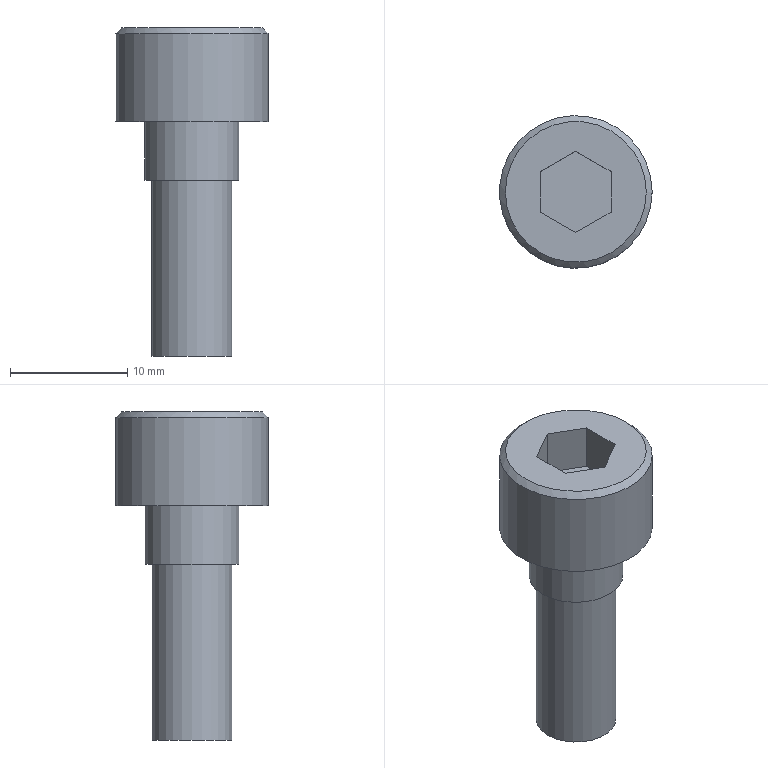Part | STEP file | M3-10_id374_x_t | 1 solid | 15 faces | box 13 x 13 x 28 mm | volume 1728 mm3 | plane 11 | cylinder 3 | cone 1 | commonest cylinder face diameters 6.8 x1 8 x1 13 x1
STEP:
#1=CARTESIAN_POINT('',(-246.986,-112.5,-17.));
#2=VERTEX_POINT('',#1);
#3=CARTESIAN_POINT('',(-243.586,-112.5,-17.));
#4=DIRECTION('',(0.,0.,-1.));
#5=DIRECTION('',(-1.,0.,0.));
#6=AXIS2_PLACEMENT_3D('',#3,#4,#5);
#7=CIRCLE('',#6,3.4);
#8=EDGE_CURVE('',#2,#2,#7,.T.);
#9=ORIENTED_EDGE('',*,*,#8,.F.);
#10=EDGE_LOOP('',(#9));
#11=FACE_BOUND('',#10,.T.);
#12=CARTESIAN_POINT('',(-239.586,-112.5,-17.));
#13=VERTEX_POINT('',#12);
#14=CARTESIAN_POINT('',(-243.586,-112.5,-17.));
#15=DIRECTION('',(0.,0.,1.));
#16=DIRECTION('',(1.,0.,0.));
#17=AXIS2_PLACEMENT_3D('',#14,#15,#16);
#18=CIRCLE('',#17,4.);
#19=EDGE_CURVE('',#13,#13,#18,.T.);
#20=ORIENTED_EDGE('',*,*,#19,.F.);
#21=EDGE_LOOP('',(#20));
#22=FACE_BOUND('',#21,.T.);
#23=CARTESIAN_POINT('',(-243.586,-112.5,-17.));
#24=DIRECTION('',(0.,0.,-1.));
#25=DIRECTION('',(-1.,0.,0.));
#26=AXIS2_PLACEMENT_3D('',#23,#24,#25);
#27=PLANE('',#26);
#28=ADVANCED_FACE('',(#11,#22),#27,.T.);
#29=CARTESIAN_POINT('',(-247.586,-112.5,-12.));
#30=VERTEX_POINT('',#29);
#31=CARTESIAN_POINT('',(-243.586,-112.5,-12.));
#32=DIRECTION('',(0.,0.,1.));
#33=DIRECTION('',(-1.,0.,0.));
#34=AXIS2_PLACEMENT_3D('',#31,#32,#33);
#35=CIRCLE('',#34,4.);
#36=EDGE_CURVE('',#30,#30,#35,.T.);
#37=ORIENTED_EDGE('',*,*,#36,.F.);
#38=EDGE_LOOP('',(#37));
#39=FACE_BOUND('',#38,.T.);
#40=ORIENTED_EDGE('',*,*,#19,.T.);
#41=EDGE_LOOP('',(#40));
#42=FACE_BOUND('',#41,.T.);
#43=CARTESIAN_POINT('',(-243.586,-112.5,-17.));
#44=DIRECTION('',(0.,0.,1.));
#45=DIRECTION('',(1.,0.,0.));
#46=AXIS2_PLACEMENT_3D('',#43,#44,#45);
#47=CYLINDRICAL_SURFACE('',#46,4.);
#48=ADVANCED_FACE('',(#39,#42),#47,.T.);
#49=CARTESIAN_POINT('',(-240.186,-112.5,-32.));
#50=VERTEX_POINT('',#49);
#51=CARTESIAN_POINT('',(-243.586,-112.5,-32.));
#52=DIRECTION('',(0.,0.,1.));
#53=DIRECTION('',(1.,0.,0.));
#54=AXIS2_PLACEMENT_3D('',#51,#52,#53);
#55=CIRCLE('',#54,3.4);
#56=EDGE_CURVE('',#50,#50,#55,.T.);
#57=ORIENTED_EDGE('',*,*,#56,.F.);
#58=EDGE_LOOP('',(#57));
#59=FACE_OUTER_BOUND('',#58,.T.);
#60=CARTESIAN_POINT('',(-243.586,-112.5,-32.));
#61=DIRECTION('',(0.,0.,-1.));
#62=DIRECTION('',(-1.,0.,0.));
#63=AXIS2_PLACEMENT_3D('',#60,#61,#62);
#64=PLANE('',#63);
#65=ADVANCED_FACE('',(#59),#64,.T.);
#66=ORIENTED_EDGE('',*,*,#56,.T.);
#67=EDGE_LOOP('',(#66));
#68=FACE_BOUND('',#67,.T.);
#69=ORIENTED_EDGE('',*,*,#8,.T.);
#70=EDGE_LOOP('',(#69));
#71=FACE_BOUND('',#70,.T.);
#72=CARTESIAN_POINT('',(-243.586,-112.5,-17.));
#73=DIRECTION('',(0.,0.,-1.));
#74=DIRECTION('',(1.,0.,0.));
#75=AXIS2_PLACEMENT_3D('',#72,#73,#74);
#76=CYLINDRICAL_SURFACE('',#75,3.4);
#77=ADVANCED_FACE('',(#68,#71),#76,.T.);
#78=CARTESIAN_POINT('',(-246.586,-110.768,-4.));
#79=VERTEX_POINT('',#78);
#80=CARTESIAN_POINT('',(-246.586,-114.232,-4.));
#81=VERTEX_POINT('',#80);
#82=CARTESIAN_POINT('',(-246.586,-110.768,-4.));
#83=DIRECTION('',(0.,-1.,0.));
#84=VECTOR('',#83,1.);
#85=LINE('',#82,#84);
#86=EDGE_CURVE('',#79,#81,#85,.T.);
#87=ORIENTED_EDGE('',*,*,#86,.F.);
#88=CARTESIAN_POINT('',(-243.586,-109.036,-4.));
#89=VERTEX_POINT('',#88);
#90=CARTESIAN_POINT('',(-243.586,-109.036,-4.));
#91=DIRECTION('',(-0.866,-0.5,0.));
#92=VECTOR('',#91,1.);
#93=LINE('',#90,#92);
#94=EDGE_CURVE('',#89,#79,#93,.T.);
#95=ORIENTED_EDGE('',*,*,#94,.F.);
#96=CARTESIAN_POINT('',(-240.586,-110.768,-4.));
#97=VERTEX_POINT('',#96);
#98=CARTESIAN_POINT('',(-240.586,-110.768,-4.));
#99=DIRECTION('',(-0.866,0.5,0.));
#100=VECTOR('',#99,1.);
#101=LINE('',#98,#100);
#102=EDGE_CURVE('',#97,#89,#101,.T.);
#103=ORIENTED_EDGE('',*,*,#102,.F.);
#104=CARTESIAN_POINT('',(-240.586,-114.232,-4.));
#105=VERTEX_POINT('',#104);
#106=CARTESIAN_POINT('',(-240.586,-114.232,-4.));
#107=DIRECTION('',(0.,1.,0.));
#108=VECTOR('',#107,1.);
#109=LINE('',#106,#108);
#110=EDGE_CURVE('',#105,#97,#109,.T.);
#111=ORIENTED_EDGE('',*,*,#110,.F.);
#112=CARTESIAN_POINT('',(-243.586,-115.964,-4.));
#113=VERTEX_POINT('',#112);
#114=CARTESIAN_POINT('',(-243.586,-115.964,-4.));
#115=DIRECTION('',(0.866,0.5,0.));
#116=VECTOR('',#115,1.);
#117=LINE('',#114,#116);
#118=EDGE_CURVE('',#113,#105,#117,.T.);
#119=ORIENTED_EDGE('',*,*,#118,.F.);
#120=CARTESIAN_POINT('',(-246.586,-114.232,-4.));
#121=DIRECTION('',(0.866,-0.5,0.));
#122=VECTOR('',#121,1.);
#123=LINE('',#120,#122);
#124=EDGE_CURVE('',#81,#113,#123,.T.);
#125=ORIENTED_EDGE('',*,*,#124,.F.);
#126=EDGE_LOOP('',(#87,#95,#103,#111,#119,#125));
#127=FACE_BOUND('',#126,.T.);
#128=CARTESIAN_POINT('',(-237.586,-112.5,-4.));
#129=VERTEX_POINT('',#128);
#130=CARTESIAN_POINT('',(-243.586,-112.5,-4.));
#131=DIRECTION('',(0.,0.,1.));
#132=DIRECTION('',(1.,0.,0.));
#133=AXIS2_PLACEMENT_3D('',#130,#131,#132);
#134=CIRCLE('',#133,6.);
#135=EDGE_CURVE('',#129,#129,#134,.T.);
#136=ORIENTED_EDGE('',*,*,#135,.T.);
#137=EDGE_LOOP('',(#136));
#138=FACE_BOUND('',#137,.T.);
#139=CARTESIAN_POINT('',(-243.586,-112.5,-4.));
#140=DIRECTION('',(0.,0.,1.));
#141=DIRECTION('',(1.,0.,0.));
#142=AXIS2_PLACEMENT_3D('',#139,#140,#141);
#143=PLANE('',#142);
#144=ADVANCED_FACE('',(#127,#138),#143,.T.);
#145=ORIENTED_EDGE('',*,*,#36,.T.);
#146=EDGE_LOOP('',(#145));
#147=FACE_BOUND('',#146,.T.);
#148=CARTESIAN_POINT('',(-237.086,-112.5,-12.));
#149=VERTEX_POINT('',#148);
#150=CARTESIAN_POINT('',(-243.586,-112.5,-12.));
#151=DIRECTION('',(0.,0.,1.));
#152=DIRECTION('',(1.,0.,0.));
#153=AXIS2_PLACEMENT_3D('',#150,#151,#152);
#154=CIRCLE('',#153,6.5);
#155=EDGE_CURVE('',#149,#149,#154,.T.);
#156=ORIENTED_EDGE('',*,*,#155,.F.);
#157=EDGE_LOOP('',(#156));
#158=FACE_BOUND('',#157,.T.);
#159=CARTESIAN_POINT('',(-243.586,-112.5,-12.));
#160=DIRECTION('',(0.,0.,-1.));
#161=DIRECTION('',(-1.,0.,0.));
#162=AXIS2_PLACEMENT_3D('',#159,#160,#161);
#163=PLANE('',#162);
#164=ADVANCED_FACE('',(#147,#158),#163,.T.);
#165=CARTESIAN_POINT('',(-237.086,-112.5,-4.5));
#166=VERTEX_POINT('',#165);
#167=CARTESIAN_POINT('',(-243.586,-112.5,-4.5));
#168=DIRECTION('',(0.,0.,-1.));
#169=DIRECTION('',(1.,0.,0.));
#170=AXIS2_PLACEMENT_3D('',#167,#168,#169);
#171=CIRCLE('',#170,6.5);
#172=EDGE_CURVE('',#166,#166,#171,.T.);
#173=ORIENTED_EDGE('',*,*,#172,.T.);
#174=EDGE_LOOP('',(#173));
#175=FACE_BOUND('',#174,.T.);
#176=ORIENTED_EDGE('',*,*,#155,.T.);
#177=EDGE_LOOP('',(#176));
#178=FACE_BOUND('',#177,.T.);
#179=CARTESIAN_POINT('',(-243.586,-112.5,-12.));
#180=DIRECTION('',(0.,0.,1.));
#181=DIRECTION('',(1.,0.,0.));
#182=AXIS2_PLACEMENT_3D('',#179,#180,#181);
#183=CYLINDRICAL_SURFACE('',#182,6.5);
#184=ADVANCED_FACE('',(#175,#178),#183,.T.);
#185=ORIENTED_EDGE('',*,*,#135,.F.);
#186=EDGE_LOOP('',(#185));
#187=FACE_BOUND('',#186,.T.);
#188=ORIENTED_EDGE('',*,*,#172,.F.);
#189=EDGE_LOOP('',(#188));
#190=FACE_BOUND('',#189,.T.);
#191=CARTESIAN_POINT('',(-243.586,-112.5,-4.5));
#192=DIRECTION('',(0.,0.,-1.));
#193=DIRECTION('',(-1.,0.,0.));
#194=AXIS2_PLACEMENT_3D('',#191,#192,#193);
#195=CONICAL_SURFACE('',#194,6.5,45.);
#196=ADVANCED_FACE('',(#187,#190),#195,.T.);
#197=ORIENTED_EDGE('',*,*,#86,.T.);
#198=CARTESIAN_POINT('',(-246.586,-114.232,-8.));
#199=VERTEX_POINT('',#198);
#200=CARTESIAN_POINT('',(-246.586,-114.232,-8.));
#201=DIRECTION('',(0.,0.,-1.));
#202=VECTOR('',#201,1.);
#203=LINE('',#200,#202);
#204=EDGE_CURVE('',#81,#199,#203,.T.);
#205=ORIENTED_EDGE('',*,*,#204,.T.);
#206=CARTESIAN_POINT('',(-246.586,-110.768,-8.));
#207=VERTEX_POINT('',#206);
#208=CARTESIAN_POINT('',(-246.586,-110.768,-8.));
#209=DIRECTION('',(0.,1.,0.));
#210=VECTOR('',#209,1.);
#211=LINE('',#208,#210);
#212=EDGE_CURVE('',#199,#207,#211,.T.);
#213=ORIENTED_EDGE('',*,*,#212,.T.);
#214=CARTESIAN_POINT('',(-246.586,-110.768,-8.));
#215=DIRECTION('',(0.,0.,-1.));
#216=VECTOR('',#215,1.);
#217=LINE('',#214,#216);
#218=EDGE_CURVE('',#79,#207,#217,.T.);
#219=ORIENTED_EDGE('',*,*,#218,.F.);
#220=EDGE_LOOP('',(#197,#205,#213,#219));
#221=FACE_OUTER_BOUND('',#220,.T.);
#222=CARTESIAN_POINT('',(-246.586,-110.768,-8.));
#223=DIRECTION('',(-1.,0.,0.));
#224=DIRECTION('',(0.,-1.,0.));
#225=AXIS2_PLACEMENT_3D('',#222,#223,#224);
#226=PLANE('',#225);
#227=ADVANCED_FACE('',(#221),#226,.F.);
#228=ORIENTED_EDGE('',*,*,#124,.T.);
#229=CARTESIAN_POINT('',(-243.586,-115.964,-8.));
#230=VERTEX_POINT('',#229);
#231=CARTESIAN_POINT('',(-243.586,-115.964,-8.));
#232=DIRECTION('',(0.,0.,-1.));
#233=VECTOR('',#232,1.);
#234=LINE('',#231,#233);
#235=EDGE_CURVE('',#113,#230,#234,.T.);
#236=ORIENTED_EDGE('',*,*,#235,.T.);
#237=CARTESIAN_POINT('',(-246.586,-114.232,-8.));
#238=DIRECTION('',(-0.866,0.5,0.));
#239=VECTOR('',#238,1.);
#240=LINE('',#237,#239);
#241=EDGE_CURVE('',#230,#199,#240,.T.);
#242=ORIENTED_EDGE('',*,*,#241,.T.);
#243=ORIENTED_EDGE('',*,*,#204,.F.);
#244=EDGE_LOOP('',(#228,#236,#242,#243));
#245=FACE_OUTER_BOUND('',#244,.T.);
#246=CARTESIAN_POINT('',(-246.586,-114.232,-8.));
#247=DIRECTION('',(-0.5,-0.866,0.));
#248=DIRECTION('',(0.866,-0.5,0.));
#249=AXIS2_PLACEMENT_3D('',#246,#247,#248);
#250=PLANE('',#249);
#251=ADVANCED_FACE('',(#245),#250,.F.);
#252=ORIENTED_EDGE('',*,*,#118,.T.);
#253=CARTESIAN_POINT('',(-240.586,-114.232,-8.));
#254=VERTEX_POINT('',#253);
#255=CARTESIAN_POINT('',(-240.586,-114.232,-8.));
#256=DIRECTION('',(0.,0.,-1.));
#257=VECTOR('',#256,1.);
#258=LINE('',#255,#257);
#259=EDGE_CURVE('',#105,#254,#258,.T.);
#260=ORIENTED_EDGE('',*,*,#259,.T.);
#261=CARTESIAN_POINT('',(-243.586,-115.964,-8.));
#262=DIRECTION('',(-0.866,-0.5,0.));
#263=VECTOR('',#262,1.);
#264=LINE('',#261,#263);
#265=EDGE_CURVE('',#254,#230,#264,.T.);
#266=ORIENTED_EDGE('',*,*,#265,.T.);
#267=ORIENTED_EDGE('',*,*,#235,.F.);
#268=EDGE_LOOP('',(#252,#260,#266,#267));
#269=FACE_OUTER_BOUND('',#268,.T.);
#270=CARTESIAN_POINT('',(-243.586,-115.964,-8.));
#271=DIRECTION('',(0.5,-0.866,0.));
#272=DIRECTION('',(0.866,0.5,0.));
#273=AXIS2_PLACEMENT_3D('',#270,#271,#272);
#274=PLANE('',#273);
#275=ADVANCED_FACE('',(#269),#274,.F.);
#276=ORIENTED_EDGE('',*,*,#110,.T.);
#277=CARTESIAN_POINT('',(-240.586,-110.768,-8.));
#278=VERTEX_POINT('',#277);
#279=CARTESIAN_POINT('',(-240.586,-110.768,-8.));
#280=DIRECTION('',(0.,0.,-1.));
#281=VECTOR('',#280,1.);
#282=LINE('',#279,#281);
#283=EDGE_CURVE('',#97,#278,#282,.T.);
#284=ORIENTED_EDGE('',*,*,#283,.T.);
#285=CARTESIAN_POINT('',(-240.586,-114.232,-8.));
#286=DIRECTION('',(0.,-1.,0.));
#287=VECTOR('',#286,1.);
#288=LINE('',#285,#287);
#289=EDGE_CURVE('',#278,#254,#288,.T.);
#290=ORIENTED_EDGE('',*,*,#289,.T.);
#291=ORIENTED_EDGE('',*,*,#259,.F.);
#292=EDGE_LOOP('',(#276,#284,#290,#291));
#293=FACE_OUTER_BOUND('',#292,.T.);
#294=CARTESIAN_POINT('',(-240.586,-114.232,-8.));
#295=DIRECTION('',(1.,0.,0.));
#296=DIRECTION('',(0.,1.,0.));
#297=AXIS2_PLACEMENT_3D('',#294,#295,#296);
#298=PLANE('',#297);
#299=ADVANCED_FACE('',(#293),#298,.F.);
#300=ORIENTED_EDGE('',*,*,#102,.T.);
#301=CARTESIAN_POINT('',(-243.586,-109.036,-8.));
#302=VERTEX_POINT('',#301);
#303=CARTESIAN_POINT('',(-243.586,-109.036,-8.));
#304=DIRECTION('',(0.,0.,-1.));
#305=VECTOR('',#304,1.);
#306=LINE('',#303,#305);
#307=EDGE_CURVE('',#89,#302,#306,.T.);
#308=ORIENTED_EDGE('',*,*,#307,.T.);
#309=CARTESIAN_POINT('',(-240.586,-110.768,-8.));
#310=DIRECTION('',(0.866,-0.5,0.));
#311=VECTOR('',#310,1.);
#312=LINE('',#309,#311);
#313=EDGE_CURVE('',#302,#278,#312,.T.);
#314=ORIENTED_EDGE('',*,*,#313,.T.);
#315=ORIENTED_EDGE('',*,*,#283,.F.);
#316=EDGE_LOOP('',(#300,#308,#314,#315));
#317=FACE_OUTER_BOUND('',#316,.T.);
#318=CARTESIAN_POINT('',(-240.586,-110.768,-8.));
#319=DIRECTION('',(0.5,0.866,0.));
#320=DIRECTION('',(-0.866,0.5,0.));
#321=AXIS2_PLACEMENT_3D('',#318,#319,#320);
#322=PLANE('',#321);
#323=ADVANCED_FACE('',(#317),#322,.F.);
#324=ORIENTED_EDGE('',*,*,#94,.T.);
#325=ORIENTED_EDGE('',*,*,#218,.T.);
#326=CARTESIAN_POINT('',(-243.586,-109.036,-8.));
#327=DIRECTION('',(0.866,0.5,0.));
#328=VECTOR('',#327,1.);
#329=LINE('',#326,#328);
#330=EDGE_CURVE('',#207,#302,#329,.T.);
#331=ORIENTED_EDGE('',*,*,#330,.T.);
#332=ORIENTED_EDGE('',*,*,#307,.F.);
#333=EDGE_LOOP('',(#324,#325,#331,#332));
#334=FACE_OUTER_BOUND('',#333,.T.);
#335=CARTESIAN_POINT('',(-243.586,-109.036,-8.));
#336=DIRECTION('',(-0.5,0.866,0.));
#337=DIRECTION('',(-0.866,-0.5,0.));
#338=AXIS2_PLACEMENT_3D('',#335,#336,#337);
#339=PLANE('',#338);
#340=ADVANCED_FACE('',(#334),#339,.F.);
#341=ORIENTED_EDGE('',*,*,#212,.F.);
#342=ORIENTED_EDGE('',*,*,#241,.F.);
#343=ORIENTED_EDGE('',*,*,#265,.F.);
#344=ORIENTED_EDGE('',*,*,#289,.F.);
#345=ORIENTED_EDGE('',*,*,#313,.F.);
#346=ORIENTED_EDGE('',*,*,#330,.F.);
#347=EDGE_LOOP('',(#341,#342,#343,#344,#345,#346));
#348=FACE_OUTER_BOUND('',#347,.T.);
#349=CARTESIAN_POINT('',(-243.586,-112.5,-8.));
#350=DIRECTION('',(0.,0.,1.));
#351=DIRECTION('',(1.,0.,0.));
#352=AXIS2_PLACEMENT_3D('',#349,#350,#351);
#353=PLANE('',#352);
#354=ADVANCED_FACE('',(#348),#353,.T.);
#355=CLOSED_SHELL('',(#28,#48,#65,#77,#144,#164,#184,#196,#227,#251,#275,#299,#323,#340,#354));
#356=MANIFOLD_SOLID_BREP('',#355);
#357=(LENGTH_UNIT()NAMED_UNIT(*)SI_UNIT(.MILLI.,.METRE.));
#358=UNCERTAINTY_MEASURE_WITH_UNIT(LENGTH_MEASURE(0.00002),#357,'','');
#359=(NAMED_UNIT(*)PLANE_ANGLE_UNIT()SI_UNIT($,.RADIAN.));
#360=PLANE_ANGLE_MEASURE_WITH_UNIT(PLANE_ANGLE_MEASURE(0.01745),#359);
#361=DIMENSIONAL_EXPONENTS(0.,0.,0.,0.,0.,0.,0.);
#362=(CONVERSION_BASED_UNIT('DEGREE',#360)NAMED_UNIT(#361)PLANE_ANGLE_UNIT());
#363=(NAMED_UNIT(*)SI_UNIT($,.STERADIAN.)SOLID_ANGLE_UNIT());
#364=(GEOMETRIC_REPRESENTATION_CONTEXT(3)GLOBAL_UNCERTAINTY_ASSIGNED_CONTEXT((#358))GLOBAL_UNIT_ASSIGNED_CONTEXT((#357,#362,#363))REPRESENTATION_CONTEXT('',''));
#365=ADVANCED_BREP_SHAPE_REPRESENTATION('',(#356),#364);